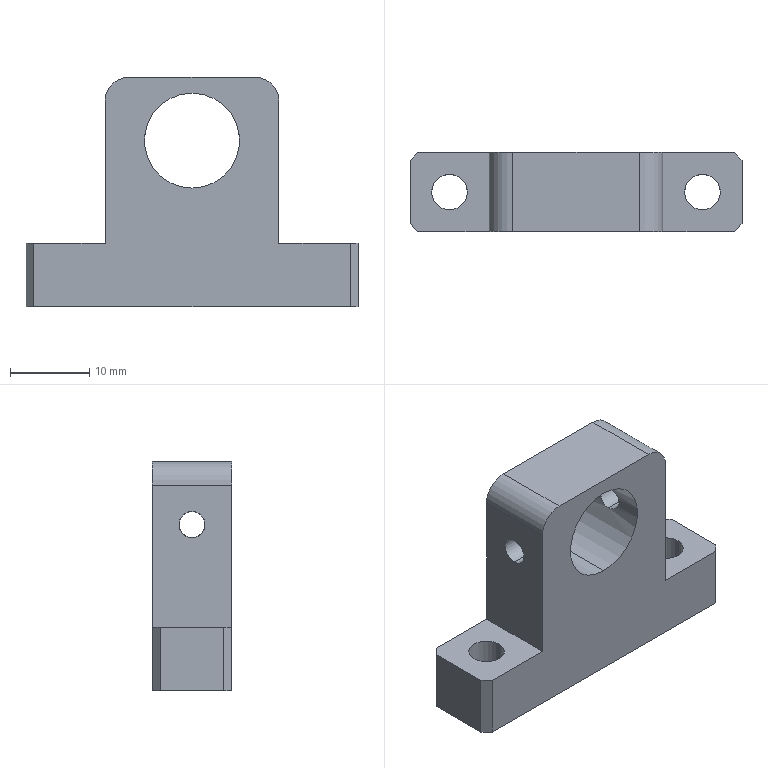Part | SolidWorks | features HoleWzd 3, ICE 3, Fillet 2, Chamfer 1, Extrusion 1 | 1 solid | 26 faces | box 42 x 10 x 29 mm | volume 6453 mm3 | plane 14 | cylinder 12 | commonest cylinder face diameters 3.3 x4 4.5 x4 6 x2 12 x2
STEP:
#1=CARTESIAN_POINT('',(-11.,0.,22.65));
#2=VERTEX_POINT('',#1);
#3=CARTESIAN_POINT('',(-11.,0.,19.35));
#4=VERTEX_POINT('',#3);
#5=CARTESIAN_POINT('',(-11.,0.,21.));
#6=DIRECTION('',(1.,0.,0.));
#7=DIRECTION('',(0.,1.,0.));
#8=AXIS2_PLACEMENT_3D('',#5,#6,#7);
#9=CIRCLE('',#8,1.65);
#10=EDGE_CURVE('',#2,#4,#9,.T.);
#11=ORIENTED_EDGE('',*,*,#10,.F.);
#12=CARTESIAN_POINT('',(-5.769,0.,22.65));
#13=VERTEX_POINT('',#12);
#14=CARTESIAN_POINT('',(11.,0.,22.65));
#15=DIRECTION('',(1.,0.,0.));
#16=VECTOR('',#15,1000.);
#17=LINE('',#14,#16);
#18=EDGE_CURVE('',#2,#13,#17,.T.);
#19=ORIENTED_EDGE('',*,*,#18,.T.);
#20=CARTESIAN_POINT('',(-5.769,0.,19.35));
#21=VERTEX_POINT('',#20);
#22=CARTESIAN_POINT('',(-5.769,0.,19.35));
#23=CARTESIAN_POINT('',(-5.769,-0.1096,19.35));
#24=CARTESIAN_POINT('',(-5.772,-0.2172,19.361));
#25=CARTESIAN_POINT('',(-5.784,-0.4288,19.403));
#26=CARTESIAN_POINT('',(-5.792,-0.5339,19.435));
#27=CARTESIAN_POINT('',(-5.814,-0.7335,19.518));
#28=CARTESIAN_POINT('',(-5.827,-0.828,19.569));
#29=CARTESIAN_POINT('',(-5.855,-1.007,19.688));
#30=CARTESIAN_POINT('',(-5.871,-1.091,19.758));
#31=CARTESIAN_POINT('',(-5.916,-1.318,19.985));
#32=CARTESIAN_POINT('',(-5.945,-1.441,20.168));
#33=CARTESIAN_POINT('',(-5.988,-1.606,20.565));
#34=CARTESIAN_POINT('',(-6.,-1.65,20.783));
#35=CARTESIAN_POINT('',(-6.,-1.65,21.108));
#36=CARTESIAN_POINT('',(-5.997,-1.639,21.217));
#37=CARTESIAN_POINT('',(-5.986,-1.597,21.43));
#38=CARTESIAN_POINT('',(-5.977,-1.565,21.533));
#39=CARTESIAN_POINT('',(-5.945,-1.441,21.833));
#40=CARTESIAN_POINT('',(-5.916,-1.319,22.015));
#41=CARTESIAN_POINT('',(-5.87,-1.09,22.243));
#42=CARTESIAN_POINT('',(-5.855,-1.007,22.311));
#43=CARTESIAN_POINT('',(-5.827,-0.8289,22.431));
#44=CARTESIAN_POINT('',(-5.814,-0.7322,22.483));
#45=CARTESIAN_POINT('',(-5.792,-0.5332,22.565));
#46=CARTESIAN_POINT('',(-5.784,-0.4303,22.597));
#47=CARTESIAN_POINT('',(-5.772,-0.2176,22.639));
#48=CARTESIAN_POINT('',(-5.769,-0.108,22.65));
#49=CARTESIAN_POINT('',(-5.769,0.,22.65));
#50=B_SPLINE_CURVE_WITH_KNOTS('',3,(#22,#23,#24,#25,#26,#27,#28,#29,#30,#31,#32,#33,#34,#35,#36,#37,#38,#39,#40,#41,#42,#43,#44,#45,#46,#47,#48,#49),.UNSPECIFIED.,.F.,.F.,(4,2,2,2,2,2,2,2,2,2,2,2,2,4),(0.,0.000324,0.000648,0.0009719,0.001296,0.001944,0.002592,0.002916,0.00324,0.003888,0.004212,0.004536,0.00486,0.005184),.UNSPECIFIED.);
#51=EDGE_CURVE('',#21,#13,#50,.T.);
#52=ORIENTED_EDGE('',*,*,#51,.F.);
#53=CARTESIAN_POINT('',(11.,0.,19.35));
#54=DIRECTION('',(1.,0.,0.));
#55=VECTOR('',#54,1000.);
#56=LINE('',#53,#55);
#57=EDGE_CURVE('',#4,#21,#56,.T.);
#58=ORIENTED_EDGE('',*,*,#57,.F.);
#59=EDGE_LOOP('',(#11,#19,#52,#58));
#60=FACE_OUTER_BOUND('',#59,.T.);
#61=CARTESIAN_POINT('',(11.,0.,21.));
#62=DIRECTION('',(1.,0.,0.));
#63=DIRECTION('',(0.,0.,-1.));
#64=AXIS2_PLACEMENT_3D('',#61,#62,#63);
#65=CYLINDRICAL_SURFACE('',#64,1.65);
#66=ADVANCED_FACE('',(#60),#65,.F.);
#67=CARTESIAN_POINT('',(5.769,0.,22.65));
#68=VERTEX_POINT('',#67);
#69=CARTESIAN_POINT('',(5.769,0.,19.35));
#70=VERTEX_POINT('',#69);
#71=CARTESIAN_POINT('',(5.769,0.,22.65));
#72=CARTESIAN_POINT('',(5.769,-0.216,22.65));
#73=CARTESIAN_POINT('',(5.782,-0.434,22.606));
#74=CARTESIAN_POINT('',(5.814,-0.7322,22.483));
#75=CARTESIAN_POINT('',(5.827,-0.8287,22.431));
#76=CARTESIAN_POINT('',(5.855,-1.007,22.311));
#77=CARTESIAN_POINT('',(5.87,-1.09,22.243));
#78=CARTESIAN_POINT('',(5.9,-1.242,22.091));
#79=CARTESIAN_POINT('',(5.916,-1.312,22.007));
#80=CARTESIAN_POINT('',(5.943,-1.431,21.829));
#81=CARTESIAN_POINT('',(5.956,-1.482,21.734));
#82=CARTESIAN_POINT('',(5.977,-1.565,21.533));
#83=CARTESIAN_POINT('',(5.986,-1.597,21.43));
#84=CARTESIAN_POINT('',(5.997,-1.639,21.218));
#85=CARTESIAN_POINT('',(6.,-1.65,21.109));
#86=CARTESIAN_POINT('',(6.,-1.65,20.892));
#87=CARTESIAN_POINT('',(5.997,-1.639,20.784));
#88=CARTESIAN_POINT('',(5.986,-1.597,20.572));
#89=CARTESIAN_POINT('',(5.977,-1.565,20.467));
#90=CARTESIAN_POINT('',(5.945,-1.441,20.168));
#91=CARTESIAN_POINT('',(5.916,-1.318,19.985));
#92=CARTESIAN_POINT('',(5.856,-1.016,19.682));
#93=CARTESIAN_POINT('',(5.825,-0.8332,19.56));
#94=CARTESIAN_POINT('',(5.793,-0.5351,19.435));
#95=CARTESIAN_POINT('',(5.784,-0.4299,19.403));
#96=CARTESIAN_POINT('',(5.772,-0.2174,19.361));
#97=CARTESIAN_POINT('',(5.769,-0.1096,19.35));
#98=CARTESIAN_POINT('',(5.769,0.,19.35));
#99=B_SPLINE_CURVE_WITH_KNOTS('',3,(#71,#72,#73,#74,#75,#76,#77,#78,#79,#80,#81,#82,#83,#84,#85,#86,#87,#88,#89,#90,#91,#92,#93,#94,#95,#96,#97,#98),.UNSPECIFIED.,.F.,.F.,(4,2,2,2,2,2,2,2,2,2,2,2,2,4),(0.005184,0.005831,0.006155,0.006479,0.006803,0.007127,0.007451,0.007775,0.008099,0.008423,0.00907,0.009718,0.01004,0.01037),.UNSPECIFIED.);
#100=EDGE_CURVE('',#68,#70,#99,.T.);
#101=ORIENTED_EDGE('',*,*,#100,.F.);
#102=CARTESIAN_POINT('',(11.,0.,22.65));
#103=VERTEX_POINT('',#102);
#104=CARTESIAN_POINT('',(11.,0.,22.65));
#105=DIRECTION('',(1.,0.,0.));
#106=VECTOR('',#105,1000.);
#107=LINE('',#104,#106);
#108=EDGE_CURVE('',#68,#103,#107,.T.);
#109=ORIENTED_EDGE('',*,*,#108,.T.);
#110=CARTESIAN_POINT('',(11.,0.,19.35));
#111=VERTEX_POINT('',#110);
#112=CARTESIAN_POINT('',(11.,0.,21.));
#113=DIRECTION('',(1.,0.,0.));
#114=DIRECTION('',(0.,0.,-1.));
#115=AXIS2_PLACEMENT_3D('',#112,#113,#114);
#116=CIRCLE('',#115,1.65);
#117=EDGE_CURVE('',#103,#111,#116,.T.);
#118=ORIENTED_EDGE('',*,*,#117,.T.);
#119=CARTESIAN_POINT('',(11.,0.,19.35));
#120=DIRECTION('',(1.,0.,0.));
#121=VECTOR('',#120,1000.);
#122=LINE('',#119,#121);
#123=EDGE_CURVE('',#70,#111,#122,.T.);
#124=ORIENTED_EDGE('',*,*,#123,.F.);
#125=EDGE_LOOP('',(#101,#109,#118,#124));
#126=FACE_OUTER_BOUND('',#125,.T.);
#127=CARTESIAN_POINT('',(11.,0.,21.));
#128=DIRECTION('',(1.,0.,0.));
#129=DIRECTION('',(0.,0.,-1.));
#130=AXIS2_PLACEMENT_3D('',#127,#128,#129);
#131=CYLINDRICAL_SURFACE('',#130,1.65);
#132=ADVANCED_FACE('',(#126),#131,.F.);
#133=CARTESIAN_POINT('',(-18.25,0.,0.));
#134=VERTEX_POINT('',#133);
#135=CARTESIAN_POINT('',(-13.75,0.,0.));
#136=VERTEX_POINT('',#135);
#137=CARTESIAN_POINT('',(-16.,0.,0.));
#138=DIRECTION('',(0.,0.,1.));
#139=DIRECTION('',(1.,0.,0.));
#140=AXIS2_PLACEMENT_3D('',#137,#138,#139);
#141=CIRCLE('',#140,2.25);
#142=EDGE_CURVE('',#134,#136,#141,.T.);
#143=ORIENTED_EDGE('',*,*,#142,.F.);
#144=CARTESIAN_POINT('',(-18.25,0.,8.));
#145=VERTEX_POINT('',#144);
#146=CARTESIAN_POINT('',(-18.25,0.,8.));
#147=DIRECTION('',(0.,0.,1.));
#148=VECTOR('',#147,1000.);
#149=LINE('',#146,#148);
#150=EDGE_CURVE('',#134,#145,#149,.T.);
#151=ORIENTED_EDGE('',*,*,#150,.T.);
#152=CARTESIAN_POINT('',(-13.75,0.,8.));
#153=VERTEX_POINT('',#152);
#154=CARTESIAN_POINT('',(-16.,0.,8.));
#155=DIRECTION('',(0.,0.,1.));
#156=DIRECTION('',(1.,0.,0.));
#157=AXIS2_PLACEMENT_3D('',#154,#155,#156);
#158=CIRCLE('',#157,2.25);
#159=EDGE_CURVE('',#145,#153,#158,.T.);
#160=ORIENTED_EDGE('',*,*,#159,.T.);
#161=CARTESIAN_POINT('',(-13.75,0.,8.));
#162=DIRECTION('',(0.,0.,1.));
#163=VECTOR('',#162,1000.);
#164=LINE('',#161,#163);
#165=EDGE_CURVE('',#136,#153,#164,.T.);
#166=ORIENTED_EDGE('',*,*,#165,.F.);
#167=EDGE_LOOP('',(#143,#151,#160,#166));
#168=FACE_OUTER_BOUND('',#167,.T.);
#169=CARTESIAN_POINT('',(-16.,0.,8.));
#170=DIRECTION('',(0.,0.,1.));
#171=DIRECTION('',(1.,0.,0.));
#172=AXIS2_PLACEMENT_3D('',#169,#170,#171);
#173=CYLINDRICAL_SURFACE('',#172,2.25);
#174=ADVANCED_FACE('',(#168),#173,.F.);
#175=CARTESIAN_POINT('',(13.75,0.,0.));
#176=VERTEX_POINT('',#175);
#177=CARTESIAN_POINT('',(18.25,0.,0.));
#178=VERTEX_POINT('',#177);
#179=CARTESIAN_POINT('',(16.,0.,0.));
#180=DIRECTION('',(0.,0.,1.));
#181=DIRECTION('',(1.,0.,0.));
#182=AXIS2_PLACEMENT_3D('',#179,#180,#181);
#183=CIRCLE('',#182,2.25);
#184=EDGE_CURVE('',#176,#178,#183,.T.);
#185=ORIENTED_EDGE('',*,*,#184,.F.);
#186=CARTESIAN_POINT('',(13.75,0.,8.));
#187=VERTEX_POINT('',#186);
#188=CARTESIAN_POINT('',(13.75,0.,8.));
#189=DIRECTION('',(0.,0.,1.));
#190=VECTOR('',#189,1000.);
#191=LINE('',#188,#190);
#192=EDGE_CURVE('',#176,#187,#191,.T.);
#193=ORIENTED_EDGE('',*,*,#192,.T.);
#194=CARTESIAN_POINT('',(18.25,0.,8.));
#195=VERTEX_POINT('',#194);
#196=CARTESIAN_POINT('',(16.,0.,8.));
#197=DIRECTION('',(0.,0.,1.));
#198=DIRECTION('',(1.,0.,0.));
#199=AXIS2_PLACEMENT_3D('',#196,#197,#198);
#200=CIRCLE('',#199,2.25);
#201=EDGE_CURVE('',#187,#195,#200,.T.);
#202=ORIENTED_EDGE('',*,*,#201,.T.);
#203=CARTESIAN_POINT('',(18.25,0.,8.));
#204=DIRECTION('',(0.,0.,1.));
#205=VECTOR('',#204,1000.);
#206=LINE('',#203,#205);
#207=EDGE_CURVE('',#178,#195,#206,.T.);
#208=ORIENTED_EDGE('',*,*,#207,.F.);
#209=EDGE_LOOP('',(#185,#193,#202,#208));
#210=FACE_OUTER_BOUND('',#209,.T.);
#211=CARTESIAN_POINT('',(16.,0.,8.));
#212=DIRECTION('',(0.,0.,1.));
#213=DIRECTION('',(1.,0.,0.));
#214=AXIS2_PLACEMENT_3D('',#211,#212,#213);
#215=CYLINDRICAL_SURFACE('',#214,2.25);
#216=ADVANCED_FACE('',(#210),#215,.F.);
#217=ORIENTED_EDGE('',*,*,#51,.T.);
#218=CARTESIAN_POINT('',(-5.769,0.,22.65));
#219=CARTESIAN_POINT('',(-5.769,0.216,22.65));
#220=CARTESIAN_POINT('',(-5.782,0.434,22.606));
#221=CARTESIAN_POINT('',(-5.814,0.7322,22.483));
#222=CARTESIAN_POINT('',(-5.827,0.8287,22.431));
#223=CARTESIAN_POINT('',(-5.855,1.007,22.311));
#224=CARTESIAN_POINT('',(-5.87,1.09,22.243));
#225=CARTESIAN_POINT('',(-5.9,1.242,22.091));
#226=CARTESIAN_POINT('',(-5.916,1.312,22.007));
#227=CARTESIAN_POINT('',(-5.943,1.431,21.829));
#228=CARTESIAN_POINT('',(-5.956,1.482,21.734));
#229=CARTESIAN_POINT('',(-5.977,1.565,21.533));
#230=CARTESIAN_POINT('',(-5.986,1.597,21.43));
#231=CARTESIAN_POINT('',(-5.997,1.639,21.218));
#232=CARTESIAN_POINT('',(-6.,1.65,21.109));
#233=CARTESIAN_POINT('',(-6.,1.65,20.892));
#234=CARTESIAN_POINT('',(-5.997,1.639,20.784));
#235=CARTESIAN_POINT('',(-5.986,1.597,20.572));
#236=CARTESIAN_POINT('',(-5.977,1.565,20.467));
#237=CARTESIAN_POINT('',(-5.945,1.441,20.168));
#238=CARTESIAN_POINT('',(-5.916,1.318,19.985));
#239=CARTESIAN_POINT('',(-5.856,1.016,19.682));
#240=CARTESIAN_POINT('',(-5.825,0.8332,19.56));
#241=CARTESIAN_POINT('',(-5.793,0.5351,19.435));
#242=CARTESIAN_POINT('',(-5.784,0.4299,19.403));
#243=CARTESIAN_POINT('',(-5.772,0.2174,19.361));
#244=CARTESIAN_POINT('',(-5.769,0.1096,19.35));
#245=CARTESIAN_POINT('',(-5.769,0.,19.35));
#246=B_SPLINE_CURVE_WITH_KNOTS('',3,(#218,#219,#220,#221,#222,#223,#224,#225,#226,#227,#228,#229,#230,#231,#232,#233,#234,#235,#236,#237,#238,#239,#240,#241,#242,#243,#244,#245),.UNSPECIFIED.,.F.,.F.,(4,2,2,2,2,2,2,2,2,2,2,2,2,4),(0.005184,0.005831,0.006155,0.006479,0.006803,0.007127,0.007451,0.007775,0.008099,0.008423,0.00907,0.009718,0.01004,0.01037),.UNSPECIFIED.);
#247=EDGE_CURVE('',#13,#21,#246,.T.);
#248=ORIENTED_EDGE('',*,*,#247,.T.);
#249=EDGE_LOOP('',(#217,#248));
#250=FACE_BOUND('',#249,.T.);
#251=CARTESIAN_POINT('',(0.,-5.,15.));
#252=VERTEX_POINT('',#251);
#253=CARTESIAN_POINT('',(0.,-5.,27.));
#254=VERTEX_POINT('',#253);
#255=CARTESIAN_POINT('',(0.,-5.,21.));
#256=DIRECTION('',(0.,1.,0.));
#257=DIRECTION('',(0.,0.,1.));
#258=AXIS2_PLACEMENT_3D('',#255,#256,#257);
#259=CIRCLE('',#258,6.);
#260=EDGE_CURVE('',#252,#254,#259,.T.);
#261=ORIENTED_EDGE('',*,*,#260,.F.);
#262=CARTESIAN_POINT('',(0.,5.,15.));
#263=VERTEX_POINT('',#262);
#264=CARTESIAN_POINT('',(0.,-5.,15.));
#265=DIRECTION('',(0.,1.,0.));
#266=VECTOR('',#265,1000.);
#267=LINE('',#264,#266);
#268=EDGE_CURVE('',#252,#263,#267,.T.);
#269=ORIENTED_EDGE('',*,*,#268,.T.);
#270=CARTESIAN_POINT('',(0.,5.,27.));
#271=VERTEX_POINT('',#270);
#272=CARTESIAN_POINT('',(0.,5.,21.));
#273=DIRECTION('',(0.,1.,0.));
#274=DIRECTION('',(0.,0.,1.));
#275=AXIS2_PLACEMENT_3D('',#272,#273,#274);
#276=CIRCLE('',#275,6.);
#277=EDGE_CURVE('',#263,#271,#276,.T.);
#278=ORIENTED_EDGE('',*,*,#277,.T.);
#279=CARTESIAN_POINT('',(0.,-5.,27.));
#280=DIRECTION('',(0.,1.,0.));
#281=VECTOR('',#280,1000.);
#282=LINE('',#279,#281);
#283=EDGE_CURVE('',#254,#271,#282,.T.);
#284=ORIENTED_EDGE('',*,*,#283,.F.);
#285=EDGE_LOOP('',(#261,#269,#278,#284));
#286=FACE_OUTER_BOUND('',#285,.T.);
#287=CARTESIAN_POINT('',(0.,-5.,21.));
#288=DIRECTION('',(0.,1.,0.));
#289=DIRECTION('',(0.,0.,1.));
#290=AXIS2_PLACEMENT_3D('',#287,#288,#289);
#291=CYLINDRICAL_SURFACE('',#290,6.);
#292=ADVANCED_FACE('',(#250,#286),#291,.F.);
#293=CARTESIAN_POINT('',(16.,0.,8.));
#294=DIRECTION('',(0.,0.,1.));
#295=DIRECTION('',(1.,0.,0.));
#296=AXIS2_PLACEMENT_3D('',#293,#294,#295);
#297=CIRCLE('',#296,2.25);
#298=EDGE_CURVE('',#195,#187,#297,.T.);
#299=ORIENTED_EDGE('',*,*,#298,.F.);
#300=ORIENTED_EDGE('',*,*,#201,.F.);
#301=EDGE_LOOP('',(#299,#300));
#302=FACE_BOUND('',#301,.T.);
#303=CARTESIAN_POINT('',(11.,-5.,8.));
#304=VERTEX_POINT('',#303);
#305=CARTESIAN_POINT('',(20.,-5.,8.));
#306=VERTEX_POINT('',#305);
#307=CARTESIAN_POINT('',(-21.,-5.,8.));
#308=DIRECTION('',(1.,0.,0.));
#309=VECTOR('',#308,1000.);
#310=LINE('',#307,#309);
#311=EDGE_CURVE('',#304,#306,#310,.T.);
#312=ORIENTED_EDGE('',*,*,#311,.T.);
#313=CARTESIAN_POINT('',(21.,-4.,8.));
#314=VERTEX_POINT('',#313);
#315=CARTESIAN_POINT('',(12.5,-12.5,8.));
#316=DIRECTION('',(0.7071,0.7071,0.));
#317=VECTOR('',#316,1000.);
#318=LINE('',#315,#317);
#319=EDGE_CURVE('',#306,#314,#318,.T.);
#320=ORIENTED_EDGE('',*,*,#319,.T.);
#321=CARTESIAN_POINT('',(21.,4.,8.));
#322=VERTEX_POINT('',#321);
#323=CARTESIAN_POINT('',(21.,5.,8.));
#324=DIRECTION('',(0.,1.,0.));
#325=VECTOR('',#324,1000.);
#326=LINE('',#323,#325);
#327=EDGE_CURVE('',#314,#322,#326,.T.);
#328=ORIENTED_EDGE('',*,*,#327,.T.);
#329=CARTESIAN_POINT('',(20.,5.,8.));
#330=VERTEX_POINT('',#329);
#331=CARTESIAN_POINT('',(12.5,12.5,8.));
#332=DIRECTION('',(-0.7071,0.7071,0.));
#333=VECTOR('',#332,1000.);
#334=LINE('',#331,#333);
#335=EDGE_CURVE('',#322,#330,#334,.T.);
#336=ORIENTED_EDGE('',*,*,#335,.T.);
#337=CARTESIAN_POINT('',(11.,5.,8.));
#338=VERTEX_POINT('',#337);
#339=CARTESIAN_POINT('',(-21.,5.,8.));
#340=DIRECTION('',(-1.,0.,0.));
#341=VECTOR('',#340,1000.);
#342=LINE('',#339,#341);
#343=EDGE_CURVE('',#330,#338,#342,.T.);
#344=ORIENTED_EDGE('',*,*,#343,.T.);
#345=CARTESIAN_POINT('',(11.,5.,8.));
#346=DIRECTION('',(0.,1.,0.));
#347=VECTOR('',#346,1000.);
#348=LINE('',#345,#347);
#349=EDGE_CURVE('',#304,#338,#348,.T.);
#350=ORIENTED_EDGE('',*,*,#349,.F.);
#351=EDGE_LOOP('',(#312,#320,#328,#336,#344,#350));
#352=FACE_OUTER_BOUND('',#351,.T.);
#353=CARTESIAN_POINT('',(0.,0.,8.));
#354=DIRECTION('',(0.,0.,1.));
#355=DIRECTION('',(1.,0.,0.));
#356=AXIS2_PLACEMENT_3D('',#353,#354,#355);
#357=PLANE('',#356);
#358=ADVANCED_FACE('',(#302,#352),#357,.T.);
#359=ORIENTED_EDGE('',*,*,#327,.F.);
#360=CARTESIAN_POINT('',(21.,-4.,0.));
#361=VERTEX_POINT('',#360);
#362=CARTESIAN_POINT('',(21.,-4.,8.));
#363=DIRECTION('',(0.,0.,-1.));
#364=VECTOR('',#363,1000.);
#365=LINE('',#362,#364);
#366=EDGE_CURVE('',#314,#361,#365,.T.);
#367=ORIENTED_EDGE('',*,*,#366,.T.);
#368=CARTESIAN_POINT('',(21.,4.,0.));
#369=VERTEX_POINT('',#368);
#370=CARTESIAN_POINT('',(21.,5.,0.));
#371=DIRECTION('',(0.,1.,0.));
#372=VECTOR('',#371,1000.);
#373=LINE('',#370,#372);
#374=EDGE_CURVE('',#361,#369,#373,.T.);
#375=ORIENTED_EDGE('',*,*,#374,.T.);
#376=CARTESIAN_POINT('',(21.,4.,8.));
#377=DIRECTION('',(0.,0.,1.));
#378=VECTOR('',#377,1000.);
#379=LINE('',#376,#378);
#380=EDGE_CURVE('',#369,#322,#379,.T.);
#381=ORIENTED_EDGE('',*,*,#380,.T.);
#382=EDGE_LOOP('',(#359,#367,#375,#381));
#383=FACE_OUTER_BOUND('',#382,.T.);
#384=CARTESIAN_POINT('',(21.,5.,8.));
#385=DIRECTION('',(-1.,0.,0.));
#386=DIRECTION('',(0.,0.,1.));
#387=AXIS2_PLACEMENT_3D('',#384,#385,#386);
#388=PLANE('',#387);
#389=ADVANCED_FACE('',(#383),#388,.F.);
#390=CARTESIAN_POINT('',(0.,5.,21.));
#391=DIRECTION('',(0.,1.,0.));
#392=DIRECTION('',(0.,0.,1.));
#393=AXIS2_PLACEMENT_3D('',#390,#391,#392);
#394=CIRCLE('',#393,6.);
#395=EDGE_CURVE('',#271,#263,#394,.T.);
#396=ORIENTED_EDGE('',*,*,#395,.F.);
#397=ORIENTED_EDGE('',*,*,#277,.F.);
#398=EDGE_LOOP('',(#396,#397));
#399=FACE_BOUND('',#398,.T.);
#400=ORIENTED_EDGE('',*,*,#343,.F.);
#401=CARTESIAN_POINT('',(20.,5.,0.));
#402=VERTEX_POINT('',#401);
#403=CARTESIAN_POINT('',(20.,5.,8.));
#404=DIRECTION('',(0.,0.,-1.));
#405=VECTOR('',#404,1000.);
#406=LINE('',#403,#405);
#407=EDGE_CURVE('',#330,#402,#406,.T.);
#408=ORIENTED_EDGE('',*,*,#407,.T.);
#409=CARTESIAN_POINT('',(-20.,5.,0.));
#410=VERTEX_POINT('',#409);
#411=CARTESIAN_POINT('',(-21.,5.,0.));
#412=DIRECTION('',(-1.,0.,0.));
#413=VECTOR('',#412,1000.);
#414=LINE('',#411,#413);
#415=EDGE_CURVE('',#402,#410,#414,.T.);
#416=ORIENTED_EDGE('',*,*,#415,.T.);
#417=CARTESIAN_POINT('',(-20.,5.,8.));
#418=VERTEX_POINT('',#417);
#419=CARTESIAN_POINT('',(-20.,5.,8.));
#420=DIRECTION('',(0.,0.,1.));
#421=VECTOR('',#420,1000.);
#422=LINE('',#419,#421);
#423=EDGE_CURVE('',#410,#418,#422,.T.);
#424=ORIENTED_EDGE('',*,*,#423,.T.);
#425=CARTESIAN_POINT('',(-11.,5.,8.));
#426=VERTEX_POINT('',#425);
#427=CARTESIAN_POINT('',(-21.,5.,8.));
#428=DIRECTION('',(-1.,0.,0.));
#429=VECTOR('',#428,1000.);
#430=LINE('',#427,#429);
#431=EDGE_CURVE('',#426,#418,#430,.T.);
#432=ORIENTED_EDGE('',*,*,#431,.F.);
#433=CARTESIAN_POINT('',(-11.,5.,26.));
#434=VERTEX_POINT('',#433);
#435=CARTESIAN_POINT('',(-11.,5.,82.166));
#436=DIRECTION('',(0.,0.,-1.));
#437=VECTOR('',#436,1000.);
#438=LINE('',#435,#437);
#439=EDGE_CURVE('',#434,#426,#438,.T.);
#440=ORIENTED_EDGE('',*,*,#439,.F.);
#441=CARTESIAN_POINT('',(-8.,5.,29.));
#442=VERTEX_POINT('',#441);
#443=CARTESIAN_POINT('',(-8.,5.,26.));
#444=DIRECTION('',(0.,1.,0.));
#445=DIRECTION('',(0.,0.,-1.));
#446=AXIS2_PLACEMENT_3D('',#443,#444,#445);
#447=CIRCLE('',#446,3.);
#448=EDGE_CURVE('',#434,#442,#447,.T.);
#449=ORIENTED_EDGE('',*,*,#448,.T.);
#450=CARTESIAN_POINT('',(8.,5.,29.));
#451=VERTEX_POINT('',#450);
#452=CARTESIAN_POINT('',(-11.,5.,29.));
#453=DIRECTION('',(-1.,0.,0.));
#454=VECTOR('',#453,1000.);
#455=LINE('',#452,#454);
#456=EDGE_CURVE('',#451,#442,#455,.T.);
#457=ORIENTED_EDGE('',*,*,#456,.F.);
#458=CARTESIAN_POINT('',(11.,5.,26.));
#459=VERTEX_POINT('',#458);
#460=CARTESIAN_POINT('',(8.,5.,26.));
#461=DIRECTION('',(0.,1.,0.));
#462=DIRECTION('',(0.,0.,-1.));
#463=AXIS2_PLACEMENT_3D('',#460,#461,#462);
#464=CIRCLE('',#463,3.);
#465=EDGE_CURVE('',#451,#459,#464,.T.);
#466=ORIENTED_EDGE('',*,*,#465,.T.);
#467=CARTESIAN_POINT('',(11.,5.,82.166));
#468=DIRECTION('',(0.,0.,-1.));
#469=VECTOR('',#468,1000.);
#470=LINE('',#467,#469);
#471=EDGE_CURVE('',#459,#338,#470,.T.);
#472=ORIENTED_EDGE('',*,*,#471,.T.);
#473=EDGE_LOOP('',(#400,#408,#416,#424,#432,#440,#449,#457,#466,#472));
#474=FACE_OUTER_BOUND('',#473,.T.);
#475=CARTESIAN_POINT('',(-21.,5.,8.));
#476=DIRECTION('',(0.,-1.,0.));
#477=DIRECTION('',(0.,0.,-1.));
#478=AXIS2_PLACEMENT_3D('',#475,#476,#477);
#479=PLANE('',#478);
#480=ADVANCED_FACE('',(#399,#474),#479,.F.);
#481=CARTESIAN_POINT('',(-21.,4.,0.));
#482=VERTEX_POINT('',#481);
#483=CARTESIAN_POINT('',(-21.,-4.,0.));
#484=VERTEX_POINT('',#483);
#485=CARTESIAN_POINT('',(-21.,5.,0.));
#486=DIRECTION('',(0.,-1.,0.));
#487=VECTOR('',#486,1000.);
#488=LINE('',#485,#487);
#489=EDGE_CURVE('',#482,#484,#488,.T.);
#490=ORIENTED_EDGE('',*,*,#489,.T.);
#491=CARTESIAN_POINT('',(-21.,-4.,8.));
#492=VERTEX_POINT('',#491);
#493=CARTESIAN_POINT('',(-21.,-4.,8.));
#494=DIRECTION('',(0.,0.,1.));
#495=VECTOR('',#494,1000.);
#496=LINE('',#493,#495);
#497=EDGE_CURVE('',#484,#492,#496,.T.);
#498=ORIENTED_EDGE('',*,*,#497,.T.);
#499=CARTESIAN_POINT('',(-21.,4.,8.));
#500=VERTEX_POINT('',#499);
#501=CARTESIAN_POINT('',(-21.,5.,8.));
#502=DIRECTION('',(0.,-1.,0.));
#503=VECTOR('',#502,1000.);
#504=LINE('',#501,#503);
#505=EDGE_CURVE('',#500,#492,#504,.T.);
#506=ORIENTED_EDGE('',*,*,#505,.F.);
#507=CARTESIAN_POINT('',(-21.,4.,8.));
#508=DIRECTION('',(0.,0.,-1.));
#509=VECTOR('',#508,1000.);
#510=LINE('',#507,#509);
#511=EDGE_CURVE('',#500,#482,#510,.T.);
#512=ORIENTED_EDGE('',*,*,#511,.T.);
#513=EDGE_LOOP('',(#490,#498,#506,#512));
#514=FACE_OUTER_BOUND('',#513,.T.);
#515=CARTESIAN_POINT('',(-21.,5.,8.));
#516=DIRECTION('',(1.,0.,0.));
#517=DIRECTION('',(0.,0.,-1.));
#518=AXIS2_PLACEMENT_3D('',#515,#516,#517);
#519=PLANE('',#518);
#520=ADVANCED_FACE('',(#514),#519,.F.);
#521=CARTESIAN_POINT('',(0.,-5.,21.));
#522=DIRECTION('',(0.,1.,0.));
#523=DIRECTION('',(0.,0.,1.));
#524=AXIS2_PLACEMENT_3D('',#521,#522,#523);
#525=CIRCLE('',#524,6.);
#526=EDGE_CURVE('',#254,#252,#525,.T.);
#527=ORIENTED_EDGE('',*,*,#526,.T.);
#528=ORIENTED_EDGE('',*,*,#260,.T.);
#529=EDGE_LOOP('',(#527,#528));
#530=FACE_BOUND('',#529,.T.);
#531=CARTESIAN_POINT('',(-20.,-5.,0.));
#532=VERTEX_POINT('',#531);
#533=CARTESIAN_POINT('',(20.,-5.,0.));
#534=VERTEX_POINT('',#533);
#535=CARTESIAN_POINT('',(-21.,-5.,0.));
#536=DIRECTION('',(1.,0.,0.));
#537=VECTOR('',#536,1000.);
#538=LINE('',#535,#537);
#539=EDGE_CURVE('',#532,#534,#538,.T.);
#540=ORIENTED_EDGE('',*,*,#539,.T.);
#541=CARTESIAN_POINT('',(20.,-5.,8.));
#542=DIRECTION('',(0.,0.,1.));
#543=VECTOR('',#542,1000.);
#544=LINE('',#541,#543);
#545=EDGE_CURVE('',#534,#306,#544,.T.);
#546=ORIENTED_EDGE('',*,*,#545,.T.);
#547=ORIENTED_EDGE('',*,*,#311,.F.);
#548=CARTESIAN_POINT('',(11.,-5.,26.));
#549=VERTEX_POINT('',#548);
#550=CARTESIAN_POINT('',(11.,-5.,82.166));
#551=DIRECTION('',(0.,0.,-1.));
#552=VECTOR('',#551,1000.);
#553=LINE('',#550,#552);
#554=EDGE_CURVE('',#549,#304,#553,.T.);
#555=ORIENTED_EDGE('',*,*,#554,.F.);
#556=CARTESIAN_POINT('',(8.,-5.,29.));
#557=VERTEX_POINT('',#556);
#558=CARTESIAN_POINT('',(8.,-5.,26.));
#559=DIRECTION('',(0.,-1.,0.));
#560=DIRECTION('',(0.,0.,1.));
#561=AXIS2_PLACEMENT_3D('',#558,#559,#560);
#562=CIRCLE('',#561,3.);
#563=EDGE_CURVE('',#549,#557,#562,.T.);
#564=ORIENTED_EDGE('',*,*,#563,.T.);
#565=CARTESIAN_POINT('',(-8.,-5.,29.));
#566=VERTEX_POINT('',#565);
#567=CARTESIAN_POINT('',(-11.,-5.,29.));
#568=DIRECTION('',(1.,0.,0.));
#569=VECTOR('',#568,1000.);
#570=LINE('',#567,#569);
#571=EDGE_CURVE('',#566,#557,#570,.T.);
#572=ORIENTED_EDGE('',*,*,#571,.F.);
#573=CARTESIAN_POINT('',(-11.,-5.,26.));
#574=VERTEX_POINT('',#573);
#575=CARTESIAN_POINT('',(-8.,-5.,26.));
#576=DIRECTION('',(0.,-1.,0.));
#577=DIRECTION('',(0.,0.,1.));
#578=AXIS2_PLACEMENT_3D('',#575,#576,#577);
#579=CIRCLE('',#578,3.);
#580=EDGE_CURVE('',#566,#574,#579,.T.);
#581=ORIENTED_EDGE('',*,*,#580,.T.);
#582=CARTESIAN_POINT('',(-11.,-5.,8.));
#583=VERTEX_POINT('',#582);
#584=CARTESIAN_POINT('',(-11.,-5.,82.166));
#585=DIRECTION('',(0.,0.,-1.));
#586=VECTOR('',#585,1000.);
#587=LINE('',#584,#586);
#588=EDGE_CURVE('',#574,#583,#587,.T.);
#589=ORIENTED_EDGE('',*,*,#588,.T.);
#590=CARTESIAN_POINT('',(-20.,-5.,8.));
#591=VERTEX_POINT('',#590);
#592=CARTESIAN_POINT('',(-21.,-5.,8.));
#593=DIRECTION('',(1.,0.,0.));
#594=VECTOR('',#593,1000.);
#595=LINE('',#592,#594);
#596=EDGE_CURVE('',#591,#583,#595,.T.);
#597=ORIENTED_EDGE('',*,*,#596,.F.);
#598=CARTESIAN_POINT('',(-20.,-5.,8.));
#599=DIRECTION('',(0.,0.,-1.));
#600=VECTOR('',#599,1000.);
#601=LINE('',#598,#600);
#602=EDGE_CURVE('',#591,#532,#601,.T.);
#603=ORIENTED_EDGE('',*,*,#602,.T.);
#604=EDGE_LOOP('',(#540,#546,#547,#555,#564,#572,#581,#589,#597,#603));
#605=FACE_OUTER_BOUND('',#604,.T.);
#606=CARTESIAN_POINT('',(-21.,-5.,8.));
#607=DIRECTION('',(0.,1.,0.));
#608=DIRECTION('',(0.,0.,1.));
#609=AXIS2_PLACEMENT_3D('',#606,#607,#608);
#610=PLANE('',#609);
#611=ADVANCED_FACE('',(#530,#605),#610,.F.);
#612=CARTESIAN_POINT('',(-16.,0.,8.));
#613=DIRECTION('',(0.,0.,1.));
#614=DIRECTION('',(1.,0.,0.));
#615=AXIS2_PLACEMENT_3D('',#612,#613,#614);
#616=CIRCLE('',#615,2.25);
#617=EDGE_CURVE('',#153,#145,#616,.T.);
#618=ORIENTED_EDGE('',*,*,#617,.F.);
#619=ORIENTED_EDGE('',*,*,#159,.F.);
#620=EDGE_LOOP('',(#618,#619));
#621=FACE_BOUND('',#620,.T.);
#622=ORIENTED_EDGE('',*,*,#505,.T.);
#623=CARTESIAN_POINT('',(-12.5,-12.5,8.));
#624=DIRECTION('',(0.7071,-0.7071,0.));
#625=VECTOR('',#624,1000.);
#626=LINE('',#623,#625);
#627=EDGE_CURVE('',#492,#591,#626,.T.);
#628=ORIENTED_EDGE('',*,*,#627,.T.);
#629=ORIENTED_EDGE('',*,*,#596,.T.);
#630=CARTESIAN_POINT('',(-11.,5.,8.));
#631=DIRECTION('',(0.,-1.,0.));
#632=VECTOR('',#631,1000.);
#633=LINE('',#630,#632);
#634=EDGE_CURVE('',#426,#583,#633,.T.);
#635=ORIENTED_EDGE('',*,*,#634,.F.);
#636=ORIENTED_EDGE('',*,*,#431,.T.);
#637=CARTESIAN_POINT('',(-12.5,12.5,8.));
#638=DIRECTION('',(-0.7071,-0.7071,0.));
#639=VECTOR('',#638,1000.);
#640=LINE('',#637,#639);
#641=EDGE_CURVE('',#418,#500,#640,.T.);
#642=ORIENTED_EDGE('',*,*,#641,.T.);
#643=EDGE_LOOP('',(#622,#628,#629,#635,#636,#642));
#644=FACE_OUTER_BOUND('',#643,.T.);
#645=CARTESIAN_POINT('',(0.,0.,8.));
#646=DIRECTION('',(0.,0.,1.));
#647=DIRECTION('',(1.,0.,0.));
#648=AXIS2_PLACEMENT_3D('',#645,#646,#647);
#649=PLANE('',#648);
#650=ADVANCED_FACE('',(#621,#644),#649,.T.);
#651=CARTESIAN_POINT('',(-16.,0.,0.));
#652=DIRECTION('',(0.,0.,1.));
#653=DIRECTION('',(1.,0.,0.));
#654=AXIS2_PLACEMENT_3D('',#651,#652,#653);
#655=CIRCLE('',#654,2.25);
#656=EDGE_CURVE('',#136,#134,#655,.T.);
#657=ORIENTED_EDGE('',*,*,#656,.T.);
#658=ORIENTED_EDGE('',*,*,#142,.T.);
#659=EDGE_LOOP('',(#657,#658));
#660=FACE_BOUND('',#659,.T.);
#661=CARTESIAN_POINT('',(16.,0.,0.));
#662=DIRECTION('',(0.,0.,1.));
#663=DIRECTION('',(1.,0.,0.));
#664=AXIS2_PLACEMENT_3D('',#661,#662,#663);
#665=CIRCLE('',#664,2.25);
#666=EDGE_CURVE('',#178,#176,#665,.T.);
#667=ORIENTED_EDGE('',*,*,#666,.T.);
#668=ORIENTED_EDGE('',*,*,#184,.T.);
#669=EDGE_LOOP('',(#667,#668));
#670=FACE_BOUND('',#669,.T.);
#671=ORIENTED_EDGE('',*,*,#374,.F.);
#672=CARTESIAN_POINT('',(21.,-4.,0.));
#673=DIRECTION('',(-0.7071,-0.7071,0.));
#674=VECTOR('',#673,1000.);
#675=LINE('',#672,#674);
#676=EDGE_CURVE('',#361,#534,#675,.T.);
#677=ORIENTED_EDGE('',*,*,#676,.T.);
#678=ORIENTED_EDGE('',*,*,#539,.F.);
#679=CARTESIAN_POINT('',(-20.,-5.,0.));
#680=DIRECTION('',(-0.7071,0.7071,0.));
#681=VECTOR('',#680,1000.);
#682=LINE('',#679,#681);
#683=EDGE_CURVE('',#532,#484,#682,.T.);
#684=ORIENTED_EDGE('',*,*,#683,.T.);
#685=ORIENTED_EDGE('',*,*,#489,.F.);
#686=CARTESIAN_POINT('',(-21.,4.,0.));
#687=DIRECTION('',(0.7071,0.7071,0.));
#688=VECTOR('',#687,1000.);
#689=LINE('',#686,#688);
#690=EDGE_CURVE('',#482,#410,#689,.T.);
#691=ORIENTED_EDGE('',*,*,#690,.T.);
#692=ORIENTED_EDGE('',*,*,#415,.F.);
#693=CARTESIAN_POINT('',(20.,5.,0.));
#694=DIRECTION('',(0.7071,-0.7071,0.));
#695=VECTOR('',#694,1000.);
#696=LINE('',#693,#695);
#697=EDGE_CURVE('',#402,#369,#696,.T.);
#698=ORIENTED_EDGE('',*,*,#697,.T.);
#699=EDGE_LOOP('',(#671,#677,#678,#684,#685,#691,#692,#698));
#700=FACE_OUTER_BOUND('',#699,.T.);
#701=CARTESIAN_POINT('',(0.,0.,0.));
#702=DIRECTION('',(0.,0.,1.));
#703=DIRECTION('',(1.,0.,0.));
#704=AXIS2_PLACEMENT_3D('',#701,#702,#703);
#705=PLANE('',#704);
#706=ADVANCED_FACE('',(#660,#670,#700),#705,.F.);
#707=CARTESIAN_POINT('',(11.,0.,21.));
#708=DIRECTION('',(1.,0.,0.));
#709=DIRECTION('',(0.,0.,-1.));
#710=AXIS2_PLACEMENT_3D('',#707,#708,#709);
#711=CIRCLE('',#710,1.65);
#712=EDGE_CURVE('',#111,#103,#711,.T.);
#713=ORIENTED_EDGE('',*,*,#712,.F.);
#714=ORIENTED_EDGE('',*,*,#117,.F.);
#715=EDGE_LOOP('',(#713,#714));
#716=FACE_BOUND('',#715,.T.);
#717=ORIENTED_EDGE('',*,*,#471,.F.);
#718=CARTESIAN_POINT('',(11.,-5.,26.));
#719=DIRECTION('',(0.,-1.,0.));
#720=VECTOR('',#719,1000.);
#721=LINE('',#718,#720);
#722=EDGE_CURVE('',#459,#549,#721,.T.);
#723=ORIENTED_EDGE('',*,*,#722,.T.);
#724=ORIENTED_EDGE('',*,*,#554,.T.);
#725=ORIENTED_EDGE('',*,*,#349,.T.);
#726=EDGE_LOOP('',(#717,#723,#724,#725));
#727=FACE_OUTER_BOUND('',#726,.T.);
#728=CARTESIAN_POINT('',(11.,5.,82.166));
#729=DIRECTION('',(-1.,0.,0.));
#730=DIRECTION('',(0.,-1.,0.));
#731=AXIS2_PLACEMENT_3D('',#728,#729,#730);
#732=PLANE('',#731);
#733=ADVANCED_FACE('',(#716,#727),#732,.F.);
#734=CARTESIAN_POINT('',(-11.,0.,21.));
#735=DIRECTION('',(1.,0.,0.));
#736=DIRECTION('',(0.,1.,0.));
#737=AXIS2_PLACEMENT_3D('',#734,#735,#736);
#738=CIRCLE('',#737,1.65);
#739=EDGE_CURVE('',#4,#2,#738,.T.);
#740=ORIENTED_EDGE('',*,*,#739,.T.);
#741=ORIENTED_EDGE('',*,*,#10,.T.);
#742=EDGE_LOOP('',(#740,#741));
#743=FACE_BOUND('',#742,.T.);
#744=ORIENTED_EDGE('',*,*,#588,.F.);
#745=CARTESIAN_POINT('',(-11.,5.,26.));
#746=DIRECTION('',(0.,1.,0.));
#747=VECTOR('',#746,1000.);
#748=LINE('',#745,#747);
#749=EDGE_CURVE('',#574,#434,#748,.T.);
#750=ORIENTED_EDGE('',*,*,#749,.T.);
#751=ORIENTED_EDGE('',*,*,#439,.T.);
#752=ORIENTED_EDGE('',*,*,#634,.T.);
#753=EDGE_LOOP('',(#744,#750,#751,#752));
#754=FACE_OUTER_BOUND('',#753,.T.);
#755=CARTESIAN_POINT('',(-11.,5.,82.166));
#756=DIRECTION('',(1.,0.,0.));
#757=DIRECTION('',(0.,1.,0.));
#758=AXIS2_PLACEMENT_3D('',#755,#756,#757);
#759=PLANE('',#758);
#760=ADVANCED_FACE('',(#743,#754),#759,.F.);
#761=ORIENTED_EDGE('',*,*,#456,.T.);
#762=CARTESIAN_POINT('',(-8.,-5.,29.));
#763=DIRECTION('',(0.,-1.,0.));
#764=VECTOR('',#763,1000.);
#765=LINE('',#762,#764);
#766=EDGE_CURVE('',#442,#566,#765,.T.);
#767=ORIENTED_EDGE('',*,*,#766,.T.);
#768=ORIENTED_EDGE('',*,*,#571,.T.);
#769=CARTESIAN_POINT('',(8.,5.,29.));
#770=DIRECTION('',(0.,1.,0.));
#771=VECTOR('',#770,1000.);
#772=LINE('',#769,#771);
#773=EDGE_CURVE('',#557,#451,#772,.T.);
#774=ORIENTED_EDGE('',*,*,#773,.T.);
#775=EDGE_LOOP('',(#761,#767,#768,#774));
#776=FACE_OUTER_BOUND('',#775,.T.);
#777=CARTESIAN_POINT('',(0.,0.,29.));
#778=DIRECTION('',(0.,0.,1.));
#779=DIRECTION('',(1.,0.,0.));
#780=AXIS2_PLACEMENT_3D('',#777,#778,#779);
#781=PLANE('',#780);
#782=ADVANCED_FACE('',(#776),#781,.T.);
#783=ORIENTED_EDGE('',*,*,#268,.F.);
#784=ORIENTED_EDGE('',*,*,#526,.F.);
#785=ORIENTED_EDGE('',*,*,#283,.T.);
#786=ORIENTED_EDGE('',*,*,#395,.T.);
#787=EDGE_LOOP('',(#783,#784,#785,#786));
#788=FACE_OUTER_BOUND('',#787,.T.);
#789=CARTESIAN_POINT('',(5.769,0.,19.35));
#790=CARTESIAN_POINT('',(5.769,0.1096,19.35));
#791=CARTESIAN_POINT('',(5.772,0.2172,19.361));
#792=CARTESIAN_POINT('',(5.784,0.4288,19.403));
#793=CARTESIAN_POINT('',(5.792,0.5339,19.435));
#794=CARTESIAN_POINT('',(5.814,0.7335,19.518));
#795=CARTESIAN_POINT('',(5.827,0.828,19.569));
#796=CARTESIAN_POINT('',(5.855,1.007,19.688));
#797=CARTESIAN_POINT('',(5.871,1.091,19.758));
#798=CARTESIAN_POINT('',(5.916,1.318,19.985));
#799=CARTESIAN_POINT('',(5.945,1.441,20.168));
#800=CARTESIAN_POINT('',(5.988,1.606,20.565));
#801=CARTESIAN_POINT('',(6.,1.65,20.783));
#802=CARTESIAN_POINT('',(6.,1.65,21.108));
#803=CARTESIAN_POINT('',(5.997,1.639,21.217));
#804=CARTESIAN_POINT('',(5.986,1.597,21.43));
#805=CARTESIAN_POINT('',(5.977,1.565,21.533));
#806=CARTESIAN_POINT('',(5.945,1.441,21.833));
#807=CARTESIAN_POINT('',(5.916,1.319,22.015));
#808=CARTESIAN_POINT('',(5.87,1.09,22.243));
#809=CARTESIAN_POINT('',(5.855,1.007,22.311));
#810=CARTESIAN_POINT('',(5.827,0.8289,22.431));
#811=CARTESIAN_POINT('',(5.814,0.7322,22.483));
#812=CARTESIAN_POINT('',(5.792,0.5332,22.565));
#813=CARTESIAN_POINT('',(5.784,0.4303,22.597));
#814=CARTESIAN_POINT('',(5.772,0.2176,22.639));
#815=CARTESIAN_POINT('',(5.769,0.108,22.65));
#816=CARTESIAN_POINT('',(5.769,0.,22.65));
#817=B_SPLINE_CURVE_WITH_KNOTS('',3,(#789,#790,#791,#792,#793,#794,#795,#796,#797,#798,#799,#800,#801,#802,#803,#804,#805,#806,#807,#808,#809,#810,#811,#812,#813,#814,#815,#816),.UNSPECIFIED.,.F.,.F.,(4,2,2,2,2,2,2,2,2,2,2,2,2,4),(0.,0.000324,0.000648,0.0009719,0.001296,0.001944,0.002592,0.002916,0.00324,0.003888,0.004212,0.004536,0.00486,0.005184),.UNSPECIFIED.);
#818=EDGE_CURVE('',#70,#68,#817,.T.);
#819=ORIENTED_EDGE('',*,*,#818,.T.);
#820=ORIENTED_EDGE('',*,*,#100,.T.);
#821=EDGE_LOOP('',(#819,#820));
#822=FACE_BOUND('',#821,.T.);
#823=CARTESIAN_POINT('',(0.,-5.,21.));
#824=DIRECTION('',(0.,1.,0.));
#825=DIRECTION('',(0.,0.,1.));
#826=AXIS2_PLACEMENT_3D('',#823,#824,#825);
#827=CYLINDRICAL_SURFACE('',#826,6.);
#828=ADVANCED_FACE('',(#788,#822),#827,.F.);
#829=ORIENTED_EDGE('',*,*,#192,.F.);
#830=ORIENTED_EDGE('',*,*,#666,.F.);
#831=ORIENTED_EDGE('',*,*,#207,.T.);
#832=ORIENTED_EDGE('',*,*,#298,.T.);
#833=EDGE_LOOP('',(#829,#830,#831,#832));
#834=FACE_OUTER_BOUND('',#833,.T.);
#835=CARTESIAN_POINT('',(16.,0.,8.));
#836=DIRECTION('',(0.,0.,1.));
#837=DIRECTION('',(1.,0.,0.));
#838=AXIS2_PLACEMENT_3D('',#835,#836,#837);
#839=CYLINDRICAL_SURFACE('',#838,2.25);
#840=ADVANCED_FACE('',(#834),#839,.F.);
#841=ORIENTED_EDGE('',*,*,#150,.F.);
#842=ORIENTED_EDGE('',*,*,#656,.F.);
#843=ORIENTED_EDGE('',*,*,#165,.T.);
#844=ORIENTED_EDGE('',*,*,#617,.T.);
#845=EDGE_LOOP('',(#841,#842,#843,#844));
#846=FACE_OUTER_BOUND('',#845,.T.);
#847=CARTESIAN_POINT('',(-16.,0.,8.));
#848=DIRECTION('',(0.,0.,1.));
#849=DIRECTION('',(1.,0.,0.));
#850=AXIS2_PLACEMENT_3D('',#847,#848,#849);
#851=CYLINDRICAL_SURFACE('',#850,2.25);
#852=ADVANCED_FACE('',(#846),#851,.F.);
#853=ORIENTED_EDGE('',*,*,#108,.F.);
#854=ORIENTED_EDGE('',*,*,#818,.F.);
#855=ORIENTED_EDGE('',*,*,#123,.T.);
#856=ORIENTED_EDGE('',*,*,#712,.T.);
#857=EDGE_LOOP('',(#853,#854,#855,#856));
#858=FACE_OUTER_BOUND('',#857,.T.);
#859=CARTESIAN_POINT('',(11.,0.,21.));
#860=DIRECTION('',(1.,0.,0.));
#861=DIRECTION('',(0.,0.,-1.));
#862=AXIS2_PLACEMENT_3D('',#859,#860,#861);
#863=CYLINDRICAL_SURFACE('',#862,1.65);
#864=ADVANCED_FACE('',(#858),#863,.F.);
#865=ORIENTED_EDGE('',*,*,#18,.F.);
#866=ORIENTED_EDGE('',*,*,#739,.F.);
#867=ORIENTED_EDGE('',*,*,#57,.T.);
#868=ORIENTED_EDGE('',*,*,#247,.F.);
#869=EDGE_LOOP('',(#865,#866,#867,#868));
#870=FACE_OUTER_BOUND('',#869,.T.);
#871=CARTESIAN_POINT('',(11.,0.,21.));
#872=DIRECTION('',(1.,0.,0.));
#873=DIRECTION('',(0.,0.,-1.));
#874=AXIS2_PLACEMENT_3D('',#871,#872,#873);
#875=CYLINDRICAL_SURFACE('',#874,1.65);
#876=ADVANCED_FACE('',(#870),#875,.F.);
#877=ORIENTED_EDGE('',*,*,#448,.F.);
#878=ORIENTED_EDGE('',*,*,#749,.F.);
#879=ORIENTED_EDGE('',*,*,#580,.F.);
#880=ORIENTED_EDGE('',*,*,#766,.F.);
#881=EDGE_LOOP('',(#877,#878,#879,#880));
#882=FACE_OUTER_BOUND('',#881,.T.);
#883=CARTESIAN_POINT('',(-8.,0.,26.));
#884=DIRECTION('',(0.,1.,0.));
#885=DIRECTION('',(-1.,0.,0.));
#886=AXIS2_PLACEMENT_3D('',#883,#884,#885);
#887=CYLINDRICAL_SURFACE('',#886,3.);
#888=ADVANCED_FACE('',(#882),#887,.T.);
#889=ORIENTED_EDGE('',*,*,#563,.F.);
#890=ORIENTED_EDGE('',*,*,#722,.F.);
#891=ORIENTED_EDGE('',*,*,#465,.F.);
#892=ORIENTED_EDGE('',*,*,#773,.F.);
#893=EDGE_LOOP('',(#889,#890,#891,#892));
#894=FACE_OUTER_BOUND('',#893,.T.);
#895=CARTESIAN_POINT('',(8.,0.,26.));
#896=DIRECTION('',(0.,-1.,0.));
#897=DIRECTION('',(1.,0.,0.));
#898=AXIS2_PLACEMENT_3D('',#895,#896,#897);
#899=CYLINDRICAL_SURFACE('',#898,3.);
#900=ADVANCED_FACE('',(#894),#899,.T.);
#901=ORIENTED_EDGE('',*,*,#319,.F.);
#902=ORIENTED_EDGE('',*,*,#545,.F.);
#903=ORIENTED_EDGE('',*,*,#676,.F.);
#904=ORIENTED_EDGE('',*,*,#366,.F.);
#905=EDGE_LOOP('',(#901,#902,#903,#904));
#906=FACE_OUTER_BOUND('',#905,.T.);
#907=CARTESIAN_POINT('',(21.,-4.,8.));
#908=DIRECTION('',(-0.7071,0.7071,0.));
#909=DIRECTION('',(0.,0.,-1.));
#910=AXIS2_PLACEMENT_3D('',#907,#908,#909);
#911=PLANE('',#910);
#912=ADVANCED_FACE('',(#906),#911,.F.);
#913=ORIENTED_EDGE('',*,*,#335,.F.);
#914=ORIENTED_EDGE('',*,*,#380,.F.);
#915=ORIENTED_EDGE('',*,*,#697,.F.);
#916=ORIENTED_EDGE('',*,*,#407,.F.);
#917=EDGE_LOOP('',(#913,#914,#915,#916));
#918=FACE_OUTER_BOUND('',#917,.T.);
#919=CARTESIAN_POINT('',(20.,5.,8.));
#920=DIRECTION('',(-0.7071,-0.7071,0.));
#921=DIRECTION('',(0.,0.,-1.));
#922=AXIS2_PLACEMENT_3D('',#919,#920,#921);
#923=PLANE('',#922);
#924=ADVANCED_FACE('',(#918),#923,.F.);
#925=ORIENTED_EDGE('',*,*,#627,.F.);
#926=ORIENTED_EDGE('',*,*,#497,.F.);
#927=ORIENTED_EDGE('',*,*,#683,.F.);
#928=ORIENTED_EDGE('',*,*,#602,.F.);
#929=EDGE_LOOP('',(#925,#926,#927,#928));
#930=FACE_OUTER_BOUND('',#929,.T.);
#931=CARTESIAN_POINT('',(-20.,-5.,8.));
#932=DIRECTION('',(0.7071,0.7071,0.));
#933=DIRECTION('',(0.,0.,-1.));
#934=AXIS2_PLACEMENT_3D('',#931,#932,#933);
#935=PLANE('',#934);
#936=ADVANCED_FACE('',(#930),#935,.F.);
#937=ORIENTED_EDGE('',*,*,#641,.F.);
#938=ORIENTED_EDGE('',*,*,#423,.F.);
#939=ORIENTED_EDGE('',*,*,#690,.F.);
#940=ORIENTED_EDGE('',*,*,#511,.F.);
#941=EDGE_LOOP('',(#937,#938,#939,#940));
#942=FACE_OUTER_BOUND('',#941,.T.);
#943=CARTESIAN_POINT('',(-21.,4.,8.));
#944=DIRECTION('',(0.7071,-0.7071,0.));
#945=DIRECTION('',(0.,0.,-1.));
#946=AXIS2_PLACEMENT_3D('',#943,#944,#945);
#947=PLANE('',#946);
#948=ADVANCED_FACE('',(#942),#947,.F.);
#949=CLOSED_SHELL('',(#66,#132,#174,#216,#292,#358,#389,#480,#520,#611,#650,#706,#733,#760,#782,#828,#840,#852,#864,#876,#888,#900,#912,#924,#936,#948));
#950=MANIFOLD_SOLID_BREP('',#949);
#951=CARTESIAN_POINT('',(0.,0.,0.));
#952=DIRECTION('',(0.,0.,1.));
#953=DIRECTION('',(1.,0.,0.));
#954=AXIS2_PLACEMENT_3D('',#951,#952,#953);
#955=(LENGTH_UNIT()NAMED_UNIT(*)SI_UNIT(.MILLI.,.METRE.));
#956=UNCERTAINTY_MEASURE_WITH_UNIT(LENGTH_MEASURE(0.00001),#955,'','');
#957=(NAMED_UNIT(*)PLANE_ANGLE_UNIT()SI_UNIT($,.RADIAN.));
#958=(NAMED_UNIT(*)SI_UNIT($,.STERADIAN.)SOLID_ANGLE_UNIT());
#959=(GEOMETRIC_REPRESENTATION_CONTEXT(3)GLOBAL_UNCERTAINTY_ASSIGNED_CONTEXT((#956))GLOBAL_UNIT_ASSIGNED_CONTEXT((#955,#957,#958))REPRESENTATION_CONTEXT('',''));
#960=ADVANCED_BREP_SHAPE_REPRESENTATION('',(#950,#954),#959);